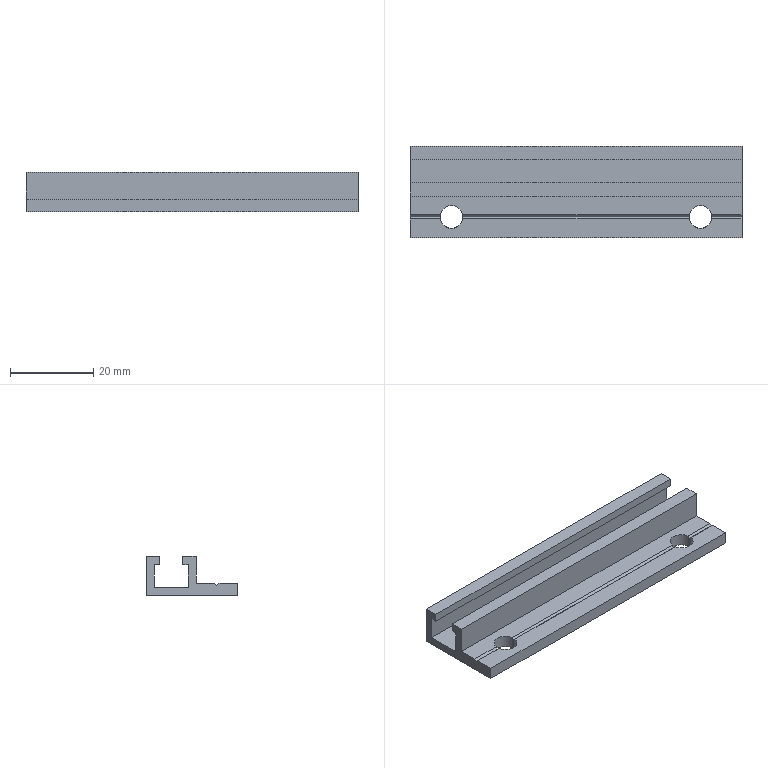Part | STEP file | SENCF5-80 | 1 solid | 27 faces | box 80 x 22 x 9.5 mm | volume 6872 mm3 | plane 23 | cylinder 4 | commonest cylinder face diameters 5.5 x4
STEP:
#1=CARTESIAN_POINT('',(72.704,-0.5,3.));
#2=VERTEX_POINT('',#1);
#3=CARTESIAN_POINT('',(72.75,0.,2.5));
#4=VERTEX_POINT('',#3);
#5=CARTESIAN_POINT('',(72.704,-0.5,3.));
#6=CARTESIAN_POINT('',(72.735,-0.335,2.835));
#7=CARTESIAN_POINT('',(72.75,-0.1678,2.668));
#8=CARTESIAN_POINT('',(72.75,0.,2.5));
#9=(BOUNDED_CURVE()B_SPLINE_CURVE(3,(#5,#6,#7,#8),.UNSPECIFIED.,.F.,.T.)B_SPLINE_CURVE_WITH_KNOTS((4,4),(4.53,4.712),.UNSPECIFIED.)CURVE()GEOMETRIC_REPRESENTATION_ITEM()RATIONAL_B_SPLINE_CURVE((1.,0.9972,0.9972,1.))REPRESENTATION_ITEM(''));
#10=EDGE_CURVE('',#2,#4,#9,.T.);
#11=ORIENTED_EDGE('',*,*,#10,.T.);
#12=CARTESIAN_POINT('',(72.75,0.,0.));
#13=VERTEX_POINT('',#12);
#14=CARTESIAN_POINT('',(72.75,0.,9.5));
#15=DIRECTION('',(0.,0.,-1.));
#16=VECTOR('',#15,1000.);
#17=LINE('',#14,#16);
#18=EDGE_CURVE('',#4,#13,#17,.T.);
#19=ORIENTED_EDGE('',*,*,#18,.T.);
#20=CARTESIAN_POINT('',(67.25,0.,0.));
#21=VERTEX_POINT('',#20);
#22=CARTESIAN_POINT('',(70.,0.,0.));
#23=DIRECTION('',(0.,0.,1.));
#24=DIRECTION('',(1.,0.,0.));
#25=AXIS2_PLACEMENT_3D('',#22,#23,#24);
#26=CIRCLE('',#25,2.75);
#27=EDGE_CURVE('',#21,#13,#26,.T.);
#28=ORIENTED_EDGE('',*,*,#27,.F.);
#29=CARTESIAN_POINT('',(67.25,0.,2.5));
#30=VERTEX_POINT('',#29);
#31=CARTESIAN_POINT('',(67.25,0.,9.5));
#32=DIRECTION('',(0.,0.,-1.));
#33=VECTOR('',#32,1000.);
#34=LINE('',#31,#33);
#35=EDGE_CURVE('',#30,#21,#34,.T.);
#36=ORIENTED_EDGE('',*,*,#35,.F.);
#37=CARTESIAN_POINT('',(67.296,-0.5,3.));
#38=VERTEX_POINT('',#37);
#39=CARTESIAN_POINT('',(67.25,0.,2.5));
#40=CARTESIAN_POINT('',(67.25,-0.1678,2.668));
#41=CARTESIAN_POINT('',(67.265,-0.335,2.835));
#42=CARTESIAN_POINT('',(67.296,-0.5,3.));
#43=(BOUNDED_CURVE()B_SPLINE_CURVE(3,(#39,#40,#41,#42),.UNSPECIFIED.,.F.,.F.)B_SPLINE_CURVE_WITH_KNOTS((4,4),(1.571,1.754),.UNSPECIFIED.)CURVE()GEOMETRIC_REPRESENTATION_ITEM()RATIONAL_B_SPLINE_CURVE((1.,0.9972,0.9972,1.))REPRESENTATION_ITEM(''));
#44=EDGE_CURVE('',#30,#38,#43,.T.);
#45=ORIENTED_EDGE('',*,*,#44,.T.);
#46=CARTESIAN_POINT('',(70.,0.,3.));
#47=DIRECTION('',(0.,0.,1.));
#48=DIRECTION('',(0.,1.,0.));
#49=AXIS2_PLACEMENT_3D('',#46,#47,#48);
#50=CIRCLE('',#49,2.75);
#51=EDGE_CURVE('',#38,#2,#50,.T.);
#52=ORIENTED_EDGE('',*,*,#51,.T.);
#53=EDGE_LOOP('',(#11,#19,#28,#36,#45,#52));
#54=FACE_OUTER_BOUND('',#53,.T.);
#55=CARTESIAN_POINT('',(70.,0.,9.5));
#56=DIRECTION('',(0.,0.,-1.));
#57=DIRECTION('',(-1.,0.,0.));
#58=AXIS2_PLACEMENT_3D('',#55,#56,#57);
#59=CYLINDRICAL_SURFACE('',#58,2.75);
#60=ADVANCED_FACE('',(#54),#59,.F.);
#61=CARTESIAN_POINT('',(12.704,-0.5,3.));
#62=VERTEX_POINT('',#61);
#63=CARTESIAN_POINT('',(12.75,0.,2.5));
#64=VERTEX_POINT('',#63);
#65=CARTESIAN_POINT('',(12.704,-0.5,3.));
#66=CARTESIAN_POINT('',(12.735,-0.335,2.835));
#67=CARTESIAN_POINT('',(12.75,-0.1678,2.668));
#68=CARTESIAN_POINT('',(12.75,0.,2.5));
#69=(BOUNDED_CURVE()B_SPLINE_CURVE(3,(#65,#66,#67,#68),.UNSPECIFIED.,.F.,.F.)B_SPLINE_CURVE_WITH_KNOTS((4,4),(4.53,4.712),.UNSPECIFIED.)CURVE()GEOMETRIC_REPRESENTATION_ITEM()RATIONAL_B_SPLINE_CURVE((1.,0.9972,0.9972,1.))REPRESENTATION_ITEM(''));
#70=EDGE_CURVE('',#62,#64,#69,.T.);
#71=ORIENTED_EDGE('',*,*,#70,.T.);
#72=CARTESIAN_POINT('',(12.75,0.,0.));
#73=VERTEX_POINT('',#72);
#74=CARTESIAN_POINT('',(12.75,0.,9.5));
#75=DIRECTION('',(0.,0.,-1.));
#76=VECTOR('',#75,1000.);
#77=LINE('',#74,#76);
#78=EDGE_CURVE('',#64,#73,#77,.T.);
#79=ORIENTED_EDGE('',*,*,#78,.T.);
#80=CARTESIAN_POINT('',(7.25,0.,0.));
#81=VERTEX_POINT('',#80);
#82=CARTESIAN_POINT('',(10.,0.,0.));
#83=DIRECTION('',(0.,0.,1.));
#84=DIRECTION('',(1.,0.,0.));
#85=AXIS2_PLACEMENT_3D('',#82,#83,#84);
#86=CIRCLE('',#85,2.75);
#87=EDGE_CURVE('',#81,#73,#86,.T.);
#88=ORIENTED_EDGE('',*,*,#87,.F.);
#89=CARTESIAN_POINT('',(7.25,0.,2.5));
#90=VERTEX_POINT('',#89);
#91=CARTESIAN_POINT('',(7.25,0.,9.5));
#92=DIRECTION('',(0.,0.,-1.));
#93=VECTOR('',#92,1000.);
#94=LINE('',#91,#93);
#95=EDGE_CURVE('',#90,#81,#94,.T.);
#96=ORIENTED_EDGE('',*,*,#95,.F.);
#97=CARTESIAN_POINT('',(7.296,-0.5,3.));
#98=VERTEX_POINT('',#97);
#99=CARTESIAN_POINT('',(7.25,0.,2.5));
#100=CARTESIAN_POINT('',(7.25,-0.1678,2.668));
#101=CARTESIAN_POINT('',(7.265,-0.335,2.835));
#102=CARTESIAN_POINT('',(7.296,-0.5,3.));
#103=(BOUNDED_CURVE()B_SPLINE_CURVE(3,(#99,#100,#101,#102),.UNSPECIFIED.,.F.,.F.)B_SPLINE_CURVE_WITH_KNOTS((4,4),(1.571,1.754),.UNSPECIFIED.)CURVE()GEOMETRIC_REPRESENTATION_ITEM()RATIONAL_B_SPLINE_CURVE((1.,0.9972,0.9972,1.))REPRESENTATION_ITEM(''));
#104=EDGE_CURVE('',#90,#98,#103,.T.);
#105=ORIENTED_EDGE('',*,*,#104,.T.);
#106=CARTESIAN_POINT('',(10.,0.,3.));
#107=DIRECTION('',(0.,0.,1.));
#108=DIRECTION('',(0.,1.,0.));
#109=AXIS2_PLACEMENT_3D('',#106,#107,#108);
#110=CIRCLE('',#109,2.75);
#111=EDGE_CURVE('',#98,#62,#110,.T.);
#112=ORIENTED_EDGE('',*,*,#111,.T.);
#113=EDGE_LOOP('',(#71,#79,#88,#96,#105,#112));
#114=FACE_OUTER_BOUND('',#113,.T.);
#115=CARTESIAN_POINT('',(10.,0.,9.5));
#116=DIRECTION('',(0.,0.,-1.));
#117=DIRECTION('',(-1.,0.,0.));
#118=AXIS2_PLACEMENT_3D('',#115,#116,#117);
#119=CYLINDRICAL_SURFACE('',#118,2.75);
#120=ADVANCED_FACE('',(#114),#119,.F.);
#121=CARTESIAN_POINT('',(0.,-5.,0.));
#122=VERTEX_POINT('',#121);
#123=CARTESIAN_POINT('',(0.,17.,0.));
#124=VERTEX_POINT('',#123);
#125=CARTESIAN_POINT('',(0.,-5.,0.));
#126=DIRECTION('',(0.,1.,0.));
#127=VECTOR('',#126,1000.);
#128=LINE('',#125,#127);
#129=EDGE_CURVE('',#122,#124,#128,.T.);
#130=ORIENTED_EDGE('',*,*,#129,.T.);
#131=CARTESIAN_POINT('',(80.,17.,0.));
#132=VERTEX_POINT('',#131);
#133=CARTESIAN_POINT('',(80.,17.,0.));
#134=DIRECTION('',(-1.,0.,0.));
#135=VECTOR('',#134,1000.);
#136=LINE('',#133,#135);
#137=EDGE_CURVE('',#132,#124,#136,.T.);
#138=ORIENTED_EDGE('',*,*,#137,.F.);
#139=CARTESIAN_POINT('',(80.,-5.,0.));
#140=VERTEX_POINT('',#139);
#141=CARTESIAN_POINT('',(80.,-5.,0.));
#142=DIRECTION('',(0.,1.,0.));
#143=VECTOR('',#142,1000.);
#144=LINE('',#141,#143);
#145=EDGE_CURVE('',#140,#132,#144,.T.);
#146=ORIENTED_EDGE('',*,*,#145,.F.);
#147=CARTESIAN_POINT('',(80.,-5.,0.));
#148=DIRECTION('',(-1.,0.,0.));
#149=VECTOR('',#148,1000.);
#150=LINE('',#147,#149);
#151=EDGE_CURVE('',#140,#122,#150,.T.);
#152=ORIENTED_EDGE('',*,*,#151,.T.);
#153=EDGE_LOOP('',(#130,#138,#146,#152));
#154=FACE_OUTER_BOUND('',#153,.T.);
#155=ORIENTED_EDGE('',*,*,#87,.T.);
#156=CARTESIAN_POINT('',(10.,0.,0.));
#157=DIRECTION('',(0.,0.,1.));
#158=DIRECTION('',(1.,0.,0.));
#159=AXIS2_PLACEMENT_3D('',#156,#157,#158);
#160=CIRCLE('',#159,2.75);
#161=EDGE_CURVE('',#73,#81,#160,.T.);
#162=ORIENTED_EDGE('',*,*,#161,.T.);
#163=EDGE_LOOP('',(#155,#162));
#164=FACE_BOUND('',#163,.T.);
#165=ORIENTED_EDGE('',*,*,#27,.T.);
#166=CARTESIAN_POINT('',(70.,0.,0.));
#167=DIRECTION('',(0.,0.,1.));
#168=DIRECTION('',(1.,0.,0.));
#169=AXIS2_PLACEMENT_3D('',#166,#167,#168);
#170=CIRCLE('',#169,2.75);
#171=EDGE_CURVE('',#13,#21,#170,.T.);
#172=ORIENTED_EDGE('',*,*,#171,.T.);
#173=EDGE_LOOP('',(#165,#172));
#174=FACE_BOUND('',#173,.T.);
#175=CARTESIAN_POINT('',(80.,-5.,0.));
#176=DIRECTION('',(0.,0.,1.));
#177=DIRECTION('',(0.,-1.,0.));
#178=AXIS2_PLACEMENT_3D('',#175,#176,#177);
#179=PLANE('',#178);
#180=ADVANCED_FACE('',(#154,#164,#174),#179,.F.);
#181=CARTESIAN_POINT('',(72.704,0.5,3.));
#182=VERTEX_POINT('',#181);
#183=CARTESIAN_POINT('',(67.296,0.5,3.));
#184=VERTEX_POINT('',#183);
#185=CARTESIAN_POINT('',(70.,0.,3.));
#186=DIRECTION('',(0.,0.,1.));
#187=DIRECTION('',(0.,1.,0.));
#188=AXIS2_PLACEMENT_3D('',#185,#186,#187);
#189=CIRCLE('',#188,2.75);
#190=EDGE_CURVE('',#182,#184,#189,.T.);
#191=ORIENTED_EDGE('',*,*,#190,.F.);
#192=CARTESIAN_POINT('',(80.,0.5,3.));
#193=VERTEX_POINT('',#192);
#194=CARTESIAN_POINT('',(80.,0.5,3.));
#195=DIRECTION('',(-1.,0.,0.));
#196=VECTOR('',#195,1000.);
#197=LINE('',#194,#196);
#198=EDGE_CURVE('',#193,#182,#197,.T.);
#199=ORIENTED_EDGE('',*,*,#198,.F.);
#200=CARTESIAN_POINT('',(80.,5.,3.));
#201=VERTEX_POINT('',#200);
#202=CARTESIAN_POINT('',(80.,5.,3.));
#203=DIRECTION('',(0.,-1.,0.));
#204=VECTOR('',#203,1000.);
#205=LINE('',#202,#204);
#206=EDGE_CURVE('',#201,#193,#205,.T.);
#207=ORIENTED_EDGE('',*,*,#206,.F.);
#208=CARTESIAN_POINT('',(0.,5.,3.));
#209=VERTEX_POINT('',#208);
#210=CARTESIAN_POINT('',(80.,5.,3.));
#211=DIRECTION('',(-1.,0.,0.));
#212=VECTOR('',#211,1000.);
#213=LINE('',#210,#212);
#214=EDGE_CURVE('',#201,#209,#213,.T.);
#215=ORIENTED_EDGE('',*,*,#214,.T.);
#216=CARTESIAN_POINT('',(0.,0.5,3.));
#217=VERTEX_POINT('',#216);
#218=CARTESIAN_POINT('',(0.,5.,3.));
#219=DIRECTION('',(0.,-1.,0.));
#220=VECTOR('',#219,1000.);
#221=LINE('',#218,#220);
#222=EDGE_CURVE('',#209,#217,#221,.T.);
#223=ORIENTED_EDGE('',*,*,#222,.T.);
#224=CARTESIAN_POINT('',(7.296,0.5,3.));
#225=VERTEX_POINT('',#224);
#226=CARTESIAN_POINT('',(80.,0.5,3.));
#227=DIRECTION('',(-1.,0.,0.));
#228=VECTOR('',#227,1000.);
#229=LINE('',#226,#228);
#230=EDGE_CURVE('',#225,#217,#229,.T.);
#231=ORIENTED_EDGE('',*,*,#230,.F.);
#232=CARTESIAN_POINT('',(12.704,0.5,3.));
#233=VERTEX_POINT('',#232);
#234=CARTESIAN_POINT('',(10.,0.,3.));
#235=DIRECTION('',(0.,0.,1.));
#236=DIRECTION('',(0.,1.,0.));
#237=AXIS2_PLACEMENT_3D('',#234,#235,#236);
#238=CIRCLE('',#237,2.75);
#239=EDGE_CURVE('',#233,#225,#238,.T.);
#240=ORIENTED_EDGE('',*,*,#239,.F.);
#241=CARTESIAN_POINT('',(80.,0.5,3.));
#242=DIRECTION('',(-1.,0.,0.));
#243=VECTOR('',#242,1000.);
#244=LINE('',#241,#243);
#245=EDGE_CURVE('',#184,#233,#244,.T.);
#246=ORIENTED_EDGE('',*,*,#245,.F.);
#247=EDGE_LOOP('',(#191,#199,#207,#215,#223,#231,#240,#246));
#248=FACE_OUTER_BOUND('',#247,.T.);
#249=CARTESIAN_POINT('',(80.,5.,3.));
#250=DIRECTION('',(0.,0.,-1.));
#251=DIRECTION('',(0.,1.,0.));
#252=AXIS2_PLACEMENT_3D('',#249,#250,#251);
#253=PLANE('',#252);
#254=ADVANCED_FACE('',(#248),#253,.F.);
#255=CARTESIAN_POINT('',(72.75,0.,2.5));
#256=CARTESIAN_POINT('',(72.75,0.1678,2.668));
#257=CARTESIAN_POINT('',(72.735,0.335,2.835));
#258=CARTESIAN_POINT('',(72.704,0.5,3.));
#259=(BOUNDED_CURVE()B_SPLINE_CURVE(3,(#255,#256,#257,#258),.UNSPECIFIED.,.F.,.F.)B_SPLINE_CURVE_WITH_KNOTS((4,4),(1.571,1.754),.UNSPECIFIED.)CURVE()GEOMETRIC_REPRESENTATION_ITEM()RATIONAL_B_SPLINE_CURVE((1.,0.9972,0.9972,1.))REPRESENTATION_ITEM(''));
#260=EDGE_CURVE('',#4,#182,#259,.T.);
#261=ORIENTED_EDGE('',*,*,#260,.F.);
#262=CARTESIAN_POINT('',(80.,0.,2.5));
#263=VERTEX_POINT('',#262);
#264=CARTESIAN_POINT('',(80.,0.,2.5));
#265=DIRECTION('',(-1.,0.,0.));
#266=VECTOR('',#265,1000.);
#267=LINE('',#264,#266);
#268=EDGE_CURVE('',#263,#4,#267,.T.);
#269=ORIENTED_EDGE('',*,*,#268,.F.);
#270=CARTESIAN_POINT('',(80.,0.5,3.));
#271=DIRECTION('',(0.,-0.7071,-0.7071));
#272=VECTOR('',#271,1000.);
#273=LINE('',#270,#272);
#274=EDGE_CURVE('',#193,#263,#273,.T.);
#275=ORIENTED_EDGE('',*,*,#274,.F.);
#276=ORIENTED_EDGE('',*,*,#198,.T.);
#277=EDGE_LOOP('',(#261,#269,#275,#276));
#278=FACE_OUTER_BOUND('',#277,.T.);
#279=CARTESIAN_POINT('',(80.,0.5,3.));
#280=DIRECTION('',(0.,0.7071,-0.7071));
#281=DIRECTION('',(0.,0.7071,0.7071));
#282=AXIS2_PLACEMENT_3D('',#279,#280,#281);
#283=PLANE('',#282);
#284=ADVANCED_FACE('',(#278),#283,.F.);
#285=CARTESIAN_POINT('',(67.296,0.5,3.));
#286=CARTESIAN_POINT('',(67.265,0.335,2.835));
#287=CARTESIAN_POINT('',(67.25,0.1678,2.668));
#288=CARTESIAN_POINT('',(67.25,0.,2.5));
#289=(BOUNDED_CURVE()B_SPLINE_CURVE(3,(#285,#286,#287,#288),.UNSPECIFIED.,.F.,.F.)B_SPLINE_CURVE_WITH_KNOTS((4,4),(4.53,4.712),.UNSPECIFIED.)CURVE()GEOMETRIC_REPRESENTATION_ITEM()RATIONAL_B_SPLINE_CURVE((1.,0.9972,0.9972,1.))REPRESENTATION_ITEM(''));
#290=EDGE_CURVE('',#184,#30,#289,.T.);
#291=ORIENTED_EDGE('',*,*,#290,.F.);
#292=ORIENTED_EDGE('',*,*,#245,.T.);
#293=CARTESIAN_POINT('',(12.75,0.,2.5));
#294=CARTESIAN_POINT('',(12.75,0.1678,2.668));
#295=CARTESIAN_POINT('',(12.735,0.335,2.835));
#296=CARTESIAN_POINT('',(12.704,0.5,3.));
#297=(BOUNDED_CURVE()B_SPLINE_CURVE(3,(#293,#294,#295,#296),.UNSPECIFIED.,.F.,.F.)B_SPLINE_CURVE_WITH_KNOTS((4,4),(1.571,1.754),.UNSPECIFIED.)CURVE()GEOMETRIC_REPRESENTATION_ITEM()RATIONAL_B_SPLINE_CURVE((1.,0.9972,0.9972,1.))REPRESENTATION_ITEM(''));
#298=EDGE_CURVE('',#64,#233,#297,.T.);
#299=ORIENTED_EDGE('',*,*,#298,.F.);
#300=CARTESIAN_POINT('',(80.,0.,2.5));
#301=DIRECTION('',(-1.,0.,0.));
#302=VECTOR('',#301,1000.);
#303=LINE('',#300,#302);
#304=EDGE_CURVE('',#30,#64,#303,.T.);
#305=ORIENTED_EDGE('',*,*,#304,.F.);
#306=EDGE_LOOP('',(#291,#292,#299,#305));
#307=FACE_OUTER_BOUND('',#306,.T.);
#308=CARTESIAN_POINT('',(80.,0.5,3.));
#309=DIRECTION('',(0.,0.7071,-0.7071));
#310=DIRECTION('',(0.,0.7071,0.7071));
#311=AXIS2_PLACEMENT_3D('',#308,#309,#310);
#312=PLANE('',#311);
#313=ADVANCED_FACE('',(#307),#312,.F.);
#314=ORIENTED_EDGE('',*,*,#44,.F.);
#315=ORIENTED_EDGE('',*,*,#304,.T.);
#316=ORIENTED_EDGE('',*,*,#70,.F.);
#317=CARTESIAN_POINT('',(80.,-0.5,3.));
#318=DIRECTION('',(-1.,0.,0.));
#319=VECTOR('',#318,1000.);
#320=LINE('',#317,#319);
#321=EDGE_CURVE('',#38,#62,#320,.T.);
#322=ORIENTED_EDGE('',*,*,#321,.F.);
#323=EDGE_LOOP('',(#314,#315,#316,#322));
#324=FACE_OUTER_BOUND('',#323,.T.);
#325=CARTESIAN_POINT('',(80.,0.,2.5));
#326=DIRECTION('',(0.,-0.7071,-0.7071));
#327=DIRECTION('',(0.,0.7071,-0.7071));
#328=AXIS2_PLACEMENT_3D('',#325,#326,#327);
#329=PLANE('',#328);
#330=ADVANCED_FACE('',(#324),#329,.F.);
#331=ORIENTED_EDGE('',*,*,#10,.F.);
#332=CARTESIAN_POINT('',(80.,-0.5,3.));
#333=VERTEX_POINT('',#332);
#334=CARTESIAN_POINT('',(80.,-0.5,3.));
#335=DIRECTION('',(-1.,0.,0.));
#336=VECTOR('',#335,1000.);
#337=LINE('',#334,#336);
#338=EDGE_CURVE('',#333,#2,#337,.T.);
#339=ORIENTED_EDGE('',*,*,#338,.F.);
#340=CARTESIAN_POINT('',(80.,0.,2.5));
#341=DIRECTION('',(0.,-0.7071,0.7071));
#342=VECTOR('',#341,1000.);
#343=LINE('',#340,#342);
#344=EDGE_CURVE('',#263,#333,#343,.T.);
#345=ORIENTED_EDGE('',*,*,#344,.F.);
#346=ORIENTED_EDGE('',*,*,#268,.T.);
#347=EDGE_LOOP('',(#331,#339,#345,#346));
#348=FACE_OUTER_BOUND('',#347,.T.);
#349=CARTESIAN_POINT('',(80.,0.,2.5));
#350=DIRECTION('',(0.,-0.7071,-0.7071));
#351=DIRECTION('',(0.,0.7071,-0.7071));
#352=AXIS2_PLACEMENT_3D('',#349,#350,#351);
#353=PLANE('',#352);
#354=ADVANCED_FACE('',(#348),#353,.F.);
#355=ORIENTED_EDGE('',*,*,#51,.F.);
#356=ORIENTED_EDGE('',*,*,#321,.T.);
#357=ORIENTED_EDGE('',*,*,#111,.F.);
#358=CARTESIAN_POINT('',(0.,-0.5,3.));
#359=VERTEX_POINT('',#358);
#360=CARTESIAN_POINT('',(80.,-0.5,3.));
#361=DIRECTION('',(-1.,0.,0.));
#362=VECTOR('',#361,1000.);
#363=LINE('',#360,#362);
#364=EDGE_CURVE('',#98,#359,#363,.T.);
#365=ORIENTED_EDGE('',*,*,#364,.T.);
#366=CARTESIAN_POINT('',(0.,-5.,3.));
#367=VERTEX_POINT('',#366);
#368=CARTESIAN_POINT('',(0.,-0.5,3.));
#369=DIRECTION('',(0.,-1.,0.));
#370=VECTOR('',#369,1000.);
#371=LINE('',#368,#370);
#372=EDGE_CURVE('',#359,#367,#371,.T.);
#373=ORIENTED_EDGE('',*,*,#372,.T.);
#374=CARTESIAN_POINT('',(80.,-5.,3.));
#375=VERTEX_POINT('',#374);
#376=CARTESIAN_POINT('',(80.,-5.,3.));
#377=DIRECTION('',(-1.,0.,0.));
#378=VECTOR('',#377,1000.);
#379=LINE('',#376,#378);
#380=EDGE_CURVE('',#375,#367,#379,.T.);
#381=ORIENTED_EDGE('',*,*,#380,.F.);
#382=CARTESIAN_POINT('',(80.,-0.5,3.));
#383=DIRECTION('',(0.,-1.,0.));
#384=VECTOR('',#383,1000.);
#385=LINE('',#382,#384);
#386=EDGE_CURVE('',#333,#375,#385,.T.);
#387=ORIENTED_EDGE('',*,*,#386,.F.);
#388=ORIENTED_EDGE('',*,*,#338,.T.);
#389=EDGE_LOOP('',(#355,#356,#357,#365,#373,#381,#387,#388));
#390=FACE_OUTER_BOUND('',#389,.T.);
#391=CARTESIAN_POINT('',(80.,-0.5,3.));
#392=DIRECTION('',(0.,0.,-1.));
#393=DIRECTION('',(0.,1.,0.));
#394=AXIS2_PLACEMENT_3D('',#391,#392,#393);
#395=PLANE('',#394);
#396=ADVANCED_FACE('',(#390),#395,.F.);
#397=CARTESIAN_POINT('',(7.296,0.5,3.));
#398=CARTESIAN_POINT('',(7.265,0.335,2.835));
#399=CARTESIAN_POINT('',(7.25,0.1678,2.668));
#400=CARTESIAN_POINT('',(7.25,0.,2.5));
#401=(BOUNDED_CURVE()B_SPLINE_CURVE(3,(#397,#398,#399,#400),.UNSPECIFIED.,.F.,.F.)B_SPLINE_CURVE_WITH_KNOTS((4,4),(4.53,4.712),.UNSPECIFIED.)CURVE()GEOMETRIC_REPRESENTATION_ITEM()RATIONAL_B_SPLINE_CURVE((1.,0.9972,0.9972,1.))REPRESENTATION_ITEM(''));
#402=EDGE_CURVE('',#225,#90,#401,.T.);
#403=ORIENTED_EDGE('',*,*,#402,.F.);
#404=ORIENTED_EDGE('',*,*,#230,.T.);
#405=CARTESIAN_POINT('',(0.,0.,2.5));
#406=VERTEX_POINT('',#405);
#407=CARTESIAN_POINT('',(0.,0.5,3.));
#408=DIRECTION('',(0.,-0.7071,-0.7071));
#409=VECTOR('',#408,1000.);
#410=LINE('',#407,#409);
#411=EDGE_CURVE('',#217,#406,#410,.T.);
#412=ORIENTED_EDGE('',*,*,#411,.T.);
#413=CARTESIAN_POINT('',(80.,0.,2.5));
#414=DIRECTION('',(-1.,0.,0.));
#415=VECTOR('',#414,1000.);
#416=LINE('',#413,#415);
#417=EDGE_CURVE('',#90,#406,#416,.T.);
#418=ORIENTED_EDGE('',*,*,#417,.F.);
#419=EDGE_LOOP('',(#403,#404,#412,#418));
#420=FACE_OUTER_BOUND('',#419,.T.);
#421=CARTESIAN_POINT('',(80.,0.5,3.));
#422=DIRECTION('',(0.,0.7071,-0.7071));
#423=DIRECTION('',(0.,0.7071,0.7071));
#424=AXIS2_PLACEMENT_3D('',#421,#422,#423);
#425=PLANE('',#424);
#426=ADVANCED_FACE('',(#420),#425,.F.);
#427=ORIENTED_EDGE('',*,*,#104,.F.);
#428=ORIENTED_EDGE('',*,*,#417,.T.);
#429=CARTESIAN_POINT('',(0.,0.,2.5));
#430=DIRECTION('',(0.,-0.7071,0.7071));
#431=VECTOR('',#430,1000.);
#432=LINE('',#429,#431);
#433=EDGE_CURVE('',#406,#359,#432,.T.);
#434=ORIENTED_EDGE('',*,*,#433,.T.);
#435=ORIENTED_EDGE('',*,*,#364,.F.);
#436=EDGE_LOOP('',(#427,#428,#434,#435));
#437=FACE_OUTER_BOUND('',#436,.T.);
#438=CARTESIAN_POINT('',(80.,0.,2.5));
#439=DIRECTION('',(0.,-0.7071,-0.7071));
#440=DIRECTION('',(0.,0.7071,-0.7071));
#441=AXIS2_PLACEMENT_3D('',#438,#439,#440);
#442=PLANE('',#441);
#443=ADVANCED_FACE('',(#437),#442,.F.);
#444=CARTESIAN_POINT('',(0.,17.,9.5));
#445=VERTEX_POINT('',#444);
#446=CARTESIAN_POINT('',(0.,17.,0.));
#447=DIRECTION('',(0.,0.,1.));
#448=VECTOR('',#447,1000.);
#449=LINE('',#446,#448);
#450=EDGE_CURVE('',#124,#445,#449,.T.);
#451=ORIENTED_EDGE('',*,*,#450,.T.);
#452=CARTESIAN_POINT('',(80.,17.,9.5));
#453=VERTEX_POINT('',#452);
#454=CARTESIAN_POINT('',(80.,17.,9.5));
#455=DIRECTION('',(-1.,0.,0.));
#456=VECTOR('',#455,1000.);
#457=LINE('',#454,#456);
#458=EDGE_CURVE('',#453,#445,#457,.T.);
#459=ORIENTED_EDGE('',*,*,#458,.F.);
#460=CARTESIAN_POINT('',(80.,17.,0.));
#461=DIRECTION('',(0.,0.,1.));
#462=VECTOR('',#461,1000.);
#463=LINE('',#460,#462);
#464=EDGE_CURVE('',#132,#453,#463,.T.);
#465=ORIENTED_EDGE('',*,*,#464,.F.);
#466=ORIENTED_EDGE('',*,*,#137,.T.);
#467=EDGE_LOOP('',(#451,#459,#465,#466));
#468=FACE_OUTER_BOUND('',#467,.T.);
#469=CARTESIAN_POINT('',(80.,17.,0.));
#470=DIRECTION('',(0.,-1.,0.));
#471=DIRECTION('',(0.,0.,-1.));
#472=AXIS2_PLACEMENT_3D('',#469,#470,#471);
#473=PLANE('',#472);
#474=ADVANCED_FACE('',(#468),#473,.F.);
#475=CARTESIAN_POINT('',(0.,13.75,9.5));
#476=VERTEX_POINT('',#475);
#477=CARTESIAN_POINT('',(0.,17.,9.5));
#478=DIRECTION('',(0.,-1.,0.));
#479=VECTOR('',#478,1000.);
#480=LINE('',#477,#479);
#481=EDGE_CURVE('',#445,#476,#480,.T.);
#482=ORIENTED_EDGE('',*,*,#481,.T.);
#483=CARTESIAN_POINT('',(80.,13.75,9.5));
#484=VERTEX_POINT('',#483);
#485=CARTESIAN_POINT('',(80.,13.75,9.5));
#486=DIRECTION('',(-1.,0.,0.));
#487=VECTOR('',#486,1000.);
#488=LINE('',#485,#487);
#489=EDGE_CURVE('',#484,#476,#488,.T.);
#490=ORIENTED_EDGE('',*,*,#489,.F.);
#491=CARTESIAN_POINT('',(80.,17.,9.5));
#492=DIRECTION('',(0.,-1.,0.));
#493=VECTOR('',#492,1000.);
#494=LINE('',#491,#493);
#495=EDGE_CURVE('',#453,#484,#494,.T.);
#496=ORIENTED_EDGE('',*,*,#495,.F.);
#497=ORIENTED_EDGE('',*,*,#458,.T.);
#498=EDGE_LOOP('',(#482,#490,#496,#497));
#499=FACE_OUTER_BOUND('',#498,.T.);
#500=CARTESIAN_POINT('',(80.,17.,9.5));
#501=DIRECTION('',(0.,0.,-1.));
#502=DIRECTION('',(0.,1.,0.));
#503=AXIS2_PLACEMENT_3D('',#500,#501,#502);
#504=PLANE('',#503);
#505=ADVANCED_FACE('',(#499),#504,.F.);
#506=CARTESIAN_POINT('',(0.,13.75,7.5));
#507=VERTEX_POINT('',#506);
#508=CARTESIAN_POINT('',(0.,13.75,9.5));
#509=DIRECTION('',(0.,0.,-1.));
#510=VECTOR('',#509,1000.);
#511=LINE('',#508,#510);
#512=EDGE_CURVE('',#476,#507,#511,.T.);
#513=ORIENTED_EDGE('',*,*,#512,.T.);
#514=CARTESIAN_POINT('',(80.,13.75,7.5));
#515=VERTEX_POINT('',#514);
#516=CARTESIAN_POINT('',(80.,13.75,7.5));
#517=DIRECTION('',(-1.,0.,0.));
#518=VECTOR('',#517,1000.);
#519=LINE('',#516,#518);
#520=EDGE_CURVE('',#515,#507,#519,.T.);
#521=ORIENTED_EDGE('',*,*,#520,.F.);
#522=CARTESIAN_POINT('',(80.,13.75,9.5));
#523=DIRECTION('',(0.,0.,-1.));
#524=VECTOR('',#523,1000.);
#525=LINE('',#522,#524);
#526=EDGE_CURVE('',#484,#515,#525,.T.);
#527=ORIENTED_EDGE('',*,*,#526,.F.);
#528=ORIENTED_EDGE('',*,*,#489,.T.);
#529=EDGE_LOOP('',(#513,#521,#527,#528));
#530=FACE_OUTER_BOUND('',#529,.T.);
#531=CARTESIAN_POINT('',(80.,13.75,9.5));
#532=DIRECTION('',(0.,1.,0.));
#533=DIRECTION('',(0.,0.,1.));
#534=AXIS2_PLACEMENT_3D('',#531,#532,#533);
#535=PLANE('',#534);
#536=ADVANCED_FACE('',(#530),#535,.F.);
#537=CARTESIAN_POINT('',(0.,15.1,7.5));
#538=VERTEX_POINT('',#537);
#539=CARTESIAN_POINT('',(0.,13.75,7.5));
#540=DIRECTION('',(0.,1.,0.));
#541=VECTOR('',#540,1000.);
#542=LINE('',#539,#541);
#543=EDGE_CURVE('',#507,#538,#542,.T.);
#544=ORIENTED_EDGE('',*,*,#543,.T.);
#545=CARTESIAN_POINT('',(80.,15.1,7.5));
#546=VERTEX_POINT('',#545);
#547=CARTESIAN_POINT('',(80.,15.1,7.5));
#548=DIRECTION('',(-1.,0.,0.));
#549=VECTOR('',#548,1000.);
#550=LINE('',#547,#549);
#551=EDGE_CURVE('',#546,#538,#550,.T.);
#552=ORIENTED_EDGE('',*,*,#551,.F.);
#553=CARTESIAN_POINT('',(80.,13.75,7.5));
#554=DIRECTION('',(0.,1.,0.));
#555=VECTOR('',#554,1000.);
#556=LINE('',#553,#555);
#557=EDGE_CURVE('',#515,#546,#556,.T.);
#558=ORIENTED_EDGE('',*,*,#557,.F.);
#559=ORIENTED_EDGE('',*,*,#520,.T.);
#560=EDGE_LOOP('',(#544,#552,#558,#559));
#561=FACE_OUTER_BOUND('',#560,.T.);
#562=CARTESIAN_POINT('',(80.,13.75,7.5));
#563=DIRECTION('',(0.,0.,1.));
#564=DIRECTION('',(1.,0.,0.));
#565=AXIS2_PLACEMENT_3D('',#562,#563,#564);
#566=PLANE('',#565);
#567=ADVANCED_FACE('',(#561),#566,.F.);
#568=CARTESIAN_POINT('',(0.,15.1,2.));
#569=VERTEX_POINT('',#568);
#570=CARTESIAN_POINT('',(0.,15.1,7.5));
#571=DIRECTION('',(0.,0.,-1.));
#572=VECTOR('',#571,1000.);
#573=LINE('',#570,#572);
#574=EDGE_CURVE('',#538,#569,#573,.T.);
#575=ORIENTED_EDGE('',*,*,#574,.T.);
#576=CARTESIAN_POINT('',(80.,15.1,2.));
#577=VERTEX_POINT('',#576);
#578=CARTESIAN_POINT('',(80.,15.1,2.));
#579=DIRECTION('',(-1.,0.,0.));
#580=VECTOR('',#579,1000.);
#581=LINE('',#578,#580);
#582=EDGE_CURVE('',#577,#569,#581,.T.);
#583=ORIENTED_EDGE('',*,*,#582,.F.);
#584=CARTESIAN_POINT('',(80.,15.1,7.5));
#585=DIRECTION('',(0.,0.,-1.));
#586=VECTOR('',#585,1000.);
#587=LINE('',#584,#586);
#588=EDGE_CURVE('',#546,#577,#587,.T.);
#589=ORIENTED_EDGE('',*,*,#588,.F.);
#590=ORIENTED_EDGE('',*,*,#551,.T.);
#591=EDGE_LOOP('',(#575,#583,#589,#590));
#592=FACE_OUTER_BOUND('',#591,.T.);
#593=CARTESIAN_POINT('',(80.,15.1,7.5));
#594=DIRECTION('',(0.,1.,0.));
#595=DIRECTION('',(0.,0.,1.));
#596=AXIS2_PLACEMENT_3D('',#593,#594,#595);
#597=PLANE('',#596);
#598=ADVANCED_FACE('',(#592),#597,.F.);
#599=CARTESIAN_POINT('',(0.,6.9,2.));
#600=VERTEX_POINT('',#599);
#601=CARTESIAN_POINT('',(0.,15.1,2.));
#602=DIRECTION('',(0.,-1.,0.));
#603=VECTOR('',#602,1000.);
#604=LINE('',#601,#603);
#605=EDGE_CURVE('',#569,#600,#604,.T.);
#606=ORIENTED_EDGE('',*,*,#605,.T.);
#607=CARTESIAN_POINT('',(80.,6.9,2.));
#608=VERTEX_POINT('',#607);
#609=CARTESIAN_POINT('',(80.,6.9,2.));
#610=DIRECTION('',(-1.,0.,0.));
#611=VECTOR('',#610,1000.);
#612=LINE('',#609,#611);
#613=EDGE_CURVE('',#608,#600,#612,.T.);
#614=ORIENTED_EDGE('',*,*,#613,.F.);
#615=CARTESIAN_POINT('',(80.,15.1,2.));
#616=DIRECTION('',(0.,-1.,0.));
#617=VECTOR('',#616,1000.);
#618=LINE('',#615,#617);
#619=EDGE_CURVE('',#577,#608,#618,.T.);
#620=ORIENTED_EDGE('',*,*,#619,.F.);
#621=ORIENTED_EDGE('',*,*,#582,.T.);
#622=EDGE_LOOP('',(#606,#614,#620,#621));
#623=FACE_OUTER_BOUND('',#622,.T.);
#624=CARTESIAN_POINT('',(80.,15.1,2.));
#625=DIRECTION('',(0.,0.,-1.));
#626=DIRECTION('',(0.,1.,0.));
#627=AXIS2_PLACEMENT_3D('',#624,#625,#626);
#628=PLANE('',#627);
#629=ADVANCED_FACE('',(#623),#628,.F.);
#630=CARTESIAN_POINT('',(0.,6.9,7.5));
#631=VERTEX_POINT('',#630);
#632=CARTESIAN_POINT('',(0.,6.9,2.));
#633=DIRECTION('',(0.,0.,1.));
#634=VECTOR('',#633,1000.);
#635=LINE('',#632,#634);
#636=EDGE_CURVE('',#600,#631,#635,.T.);
#637=ORIENTED_EDGE('',*,*,#636,.T.);
#638=CARTESIAN_POINT('',(80.,6.9,7.5));
#639=VERTEX_POINT('',#638);
#640=CARTESIAN_POINT('',(80.,6.9,7.5));
#641=DIRECTION('',(-1.,0.,0.));
#642=VECTOR('',#641,1000.);
#643=LINE('',#640,#642);
#644=EDGE_CURVE('',#639,#631,#643,.T.);
#645=ORIENTED_EDGE('',*,*,#644,.F.);
#646=CARTESIAN_POINT('',(80.,6.9,2.));
#647=DIRECTION('',(0.,0.,1.));
#648=VECTOR('',#647,1000.);
#649=LINE('',#646,#648);
#650=EDGE_CURVE('',#608,#639,#649,.T.);
#651=ORIENTED_EDGE('',*,*,#650,.F.);
#652=ORIENTED_EDGE('',*,*,#613,.T.);
#653=EDGE_LOOP('',(#637,#645,#651,#652));
#654=FACE_OUTER_BOUND('',#653,.T.);
#655=CARTESIAN_POINT('',(80.,6.9,2.));
#656=DIRECTION('',(0.,-1.,0.));
#657=DIRECTION('',(0.,0.,-1.));
#658=AXIS2_PLACEMENT_3D('',#655,#656,#657);
#659=PLANE('',#658);
#660=ADVANCED_FACE('',(#654),#659,.F.);
#661=CARTESIAN_POINT('',(0.,8.25,7.5));
#662=VERTEX_POINT('',#661);
#663=CARTESIAN_POINT('',(0.,6.9,7.5));
#664=DIRECTION('',(0.,1.,0.));
#665=VECTOR('',#664,1000.);
#666=LINE('',#663,#665);
#667=EDGE_CURVE('',#631,#662,#666,.T.);
#668=ORIENTED_EDGE('',*,*,#667,.T.);
#669=CARTESIAN_POINT('',(80.,8.25,7.5));
#670=VERTEX_POINT('',#669);
#671=CARTESIAN_POINT('',(80.,8.25,7.5));
#672=DIRECTION('',(-1.,0.,0.));
#673=VECTOR('',#672,1000.);
#674=LINE('',#671,#673);
#675=EDGE_CURVE('',#670,#662,#674,.T.);
#676=ORIENTED_EDGE('',*,*,#675,.F.);
#677=CARTESIAN_POINT('',(80.,6.9,7.5));
#678=DIRECTION('',(0.,1.,0.));
#679=VECTOR('',#678,1000.);
#680=LINE('',#677,#679);
#681=EDGE_CURVE('',#639,#670,#680,.T.);
#682=ORIENTED_EDGE('',*,*,#681,.F.);
#683=ORIENTED_EDGE('',*,*,#644,.T.);
#684=EDGE_LOOP('',(#668,#676,#682,#683));
#685=FACE_OUTER_BOUND('',#684,.T.);
#686=CARTESIAN_POINT('',(80.,6.9,7.5));
#687=DIRECTION('',(0.,0.,1.));
#688=DIRECTION('',(1.,0.,0.));
#689=AXIS2_PLACEMENT_3D('',#686,#687,#688);
#690=PLANE('',#689);
#691=ADVANCED_FACE('',(#685),#690,.F.);
#692=CARTESIAN_POINT('',(0.,8.25,9.5));
#693=VERTEX_POINT('',#692);
#694=CARTESIAN_POINT('',(0.,8.25,7.5));
#695=DIRECTION('',(0.,0.,1.));
#696=VECTOR('',#695,1000.);
#697=LINE('',#694,#696);
#698=EDGE_CURVE('',#662,#693,#697,.T.);
#699=ORIENTED_EDGE('',*,*,#698,.T.);
#700=CARTESIAN_POINT('',(80.,8.25,9.5));
#701=VERTEX_POINT('',#700);
#702=CARTESIAN_POINT('',(80.,8.25,9.5));
#703=DIRECTION('',(-1.,0.,0.));
#704=VECTOR('',#703,1000.);
#705=LINE('',#702,#704);
#706=EDGE_CURVE('',#701,#693,#705,.T.);
#707=ORIENTED_EDGE('',*,*,#706,.F.);
#708=CARTESIAN_POINT('',(80.,8.25,7.5));
#709=DIRECTION('',(0.,0.,1.));
#710=VECTOR('',#709,1000.);
#711=LINE('',#708,#710);
#712=EDGE_CURVE('',#670,#701,#711,.T.);
#713=ORIENTED_EDGE('',*,*,#712,.F.);
#714=ORIENTED_EDGE('',*,*,#675,.T.);
#715=EDGE_LOOP('',(#699,#707,#713,#714));
#716=FACE_OUTER_BOUND('',#715,.T.);
#717=CARTESIAN_POINT('',(80.,8.25,7.5));
#718=DIRECTION('',(0.,-1.,0.));
#719=DIRECTION('',(0.,0.,-1.));
#720=AXIS2_PLACEMENT_3D('',#717,#718,#719);
#721=PLANE('',#720);
#722=ADVANCED_FACE('',(#716),#721,.F.);
#723=CARTESIAN_POINT('',(0.,5.,9.5));
#724=VERTEX_POINT('',#723);
#725=CARTESIAN_POINT('',(0.,8.25,9.5));
#726=DIRECTION('',(0.,-1.,0.));
#727=VECTOR('',#726,1000.);
#728=LINE('',#725,#727);
#729=EDGE_CURVE('',#693,#724,#728,.T.);
#730=ORIENTED_EDGE('',*,*,#729,.T.);
#731=CARTESIAN_POINT('',(80.,5.,9.5));
#732=VERTEX_POINT('',#731);
#733=CARTESIAN_POINT('',(80.,5.,9.5));
#734=DIRECTION('',(-1.,0.,0.));
#735=VECTOR('',#734,1000.);
#736=LINE('',#733,#735);
#737=EDGE_CURVE('',#732,#724,#736,.T.);
#738=ORIENTED_EDGE('',*,*,#737,.F.);
#739=CARTESIAN_POINT('',(80.,8.25,9.5));
#740=DIRECTION('',(0.,-1.,0.));
#741=VECTOR('',#740,1000.);
#742=LINE('',#739,#741);
#743=EDGE_CURVE('',#701,#732,#742,.T.);
#744=ORIENTED_EDGE('',*,*,#743,.F.);
#745=ORIENTED_EDGE('',*,*,#706,.T.);
#746=EDGE_LOOP('',(#730,#738,#744,#745));
#747=FACE_OUTER_BOUND('',#746,.T.);
#748=CARTESIAN_POINT('',(80.,8.25,9.5));
#749=DIRECTION('',(0.,0.,-1.));
#750=DIRECTION('',(-1.,0.,0.));
#751=AXIS2_PLACEMENT_3D('',#748,#749,#750);
#752=PLANE('',#751);
#753=ADVANCED_FACE('',(#747),#752,.F.);
#754=CARTESIAN_POINT('',(0.,5.,9.5));
#755=DIRECTION('',(0.,0.,-1.));
#756=VECTOR('',#755,1000.);
#757=LINE('',#754,#756);
#758=EDGE_CURVE('',#724,#209,#757,.T.);
#759=ORIENTED_EDGE('',*,*,#758,.T.);
#760=ORIENTED_EDGE('',*,*,#214,.F.);
#761=CARTESIAN_POINT('',(80.,5.,9.5));
#762=DIRECTION('',(0.,0.,-1.));
#763=VECTOR('',#762,1000.);
#764=LINE('',#761,#763);
#765=EDGE_CURVE('',#732,#201,#764,.T.);
#766=ORIENTED_EDGE('',*,*,#765,.F.);
#767=ORIENTED_EDGE('',*,*,#737,.T.);
#768=EDGE_LOOP('',(#759,#760,#766,#767));
#769=FACE_OUTER_BOUND('',#768,.T.);
#770=CARTESIAN_POINT('',(80.,5.,9.5));
#771=DIRECTION('',(0.,1.,0.));
#772=DIRECTION('',(0.,0.,1.));
#773=AXIS2_PLACEMENT_3D('',#770,#771,#772);
#774=PLANE('',#773);
#775=ADVANCED_FACE('',(#769),#774,.F.);
#776=CARTESIAN_POINT('',(0.,-5.,3.));
#777=DIRECTION('',(0.,0.,-1.));
#778=VECTOR('',#777,1000.);
#779=LINE('',#776,#778);
#780=EDGE_CURVE('',#367,#122,#779,.T.);
#781=ORIENTED_EDGE('',*,*,#780,.T.);
#782=ORIENTED_EDGE('',*,*,#151,.F.);
#783=CARTESIAN_POINT('',(80.,-5.,3.));
#784=DIRECTION('',(0.,0.,-1.));
#785=VECTOR('',#784,1000.);
#786=LINE('',#783,#785);
#787=EDGE_CURVE('',#375,#140,#786,.T.);
#788=ORIENTED_EDGE('',*,*,#787,.F.);
#789=ORIENTED_EDGE('',*,*,#380,.T.);
#790=EDGE_LOOP('',(#781,#782,#788,#789));
#791=FACE_OUTER_BOUND('',#790,.T.);
#792=CARTESIAN_POINT('',(80.,-5.,3.));
#793=DIRECTION('',(0.,1.,0.));
#794=DIRECTION('',(0.,0.,1.));
#795=AXIS2_PLACEMENT_3D('',#792,#793,#794);
#796=PLANE('',#795);
#797=ADVANCED_FACE('',(#791),#796,.F.);
#798=ORIENTED_EDGE('',*,*,#145,.T.);
#799=ORIENTED_EDGE('',*,*,#464,.T.);
#800=ORIENTED_EDGE('',*,*,#495,.T.);
#801=ORIENTED_EDGE('',*,*,#526,.T.);
#802=ORIENTED_EDGE('',*,*,#557,.T.);
#803=ORIENTED_EDGE('',*,*,#588,.T.);
#804=ORIENTED_EDGE('',*,*,#619,.T.);
#805=ORIENTED_EDGE('',*,*,#650,.T.);
#806=ORIENTED_EDGE('',*,*,#681,.T.);
#807=ORIENTED_EDGE('',*,*,#712,.T.);
#808=ORIENTED_EDGE('',*,*,#743,.T.);
#809=ORIENTED_EDGE('',*,*,#765,.T.);
#810=ORIENTED_EDGE('',*,*,#206,.T.);
#811=ORIENTED_EDGE('',*,*,#274,.T.);
#812=ORIENTED_EDGE('',*,*,#344,.T.);
#813=ORIENTED_EDGE('',*,*,#386,.T.);
#814=ORIENTED_EDGE('',*,*,#787,.T.);
#815=EDGE_LOOP('',(#798,#799,#800,#801,#802,#803,#804,#805,#806,#807,#808,#809,#810,#811,#812,#813,#814));
#816=FACE_OUTER_BOUND('',#815,.T.);
#817=CARTESIAN_POINT('',(80.,0.,0.));
#818=DIRECTION('',(1.,0.,0.));
#819=DIRECTION('',(0.,0.,-1.));
#820=AXIS2_PLACEMENT_3D('',#817,#818,#819);
#821=PLANE('',#820);
#822=ADVANCED_FACE('',(#816),#821,.T.);
#823=ORIENTED_EDGE('',*,*,#129,.F.);
#824=ORIENTED_EDGE('',*,*,#780,.F.);
#825=ORIENTED_EDGE('',*,*,#372,.F.);
#826=ORIENTED_EDGE('',*,*,#433,.F.);
#827=ORIENTED_EDGE('',*,*,#411,.F.);
#828=ORIENTED_EDGE('',*,*,#222,.F.);
#829=ORIENTED_EDGE('',*,*,#758,.F.);
#830=ORIENTED_EDGE('',*,*,#729,.F.);
#831=ORIENTED_EDGE('',*,*,#698,.F.);
#832=ORIENTED_EDGE('',*,*,#667,.F.);
#833=ORIENTED_EDGE('',*,*,#636,.F.);
#834=ORIENTED_EDGE('',*,*,#605,.F.);
#835=ORIENTED_EDGE('',*,*,#574,.F.);
#836=ORIENTED_EDGE('',*,*,#543,.F.);
#837=ORIENTED_EDGE('',*,*,#512,.F.);
#838=ORIENTED_EDGE('',*,*,#481,.F.);
#839=ORIENTED_EDGE('',*,*,#450,.F.);
#840=EDGE_LOOP('',(#823,#824,#825,#826,#827,#828,#829,#830,#831,#832,#833,#834,#835,#836,#837,#838,#839));
#841=FACE_OUTER_BOUND('',#840,.T.);
#842=CARTESIAN_POINT('',(0.,0.,0.));
#843=DIRECTION('',(1.,0.,0.));
#844=DIRECTION('',(0.,0.,-1.));
#845=AXIS2_PLACEMENT_3D('',#842,#843,#844);
#846=PLANE('',#845);
#847=ADVANCED_FACE('',(#841),#846,.F.);
#848=ORIENTED_EDGE('',*,*,#78,.F.);
#849=ORIENTED_EDGE('',*,*,#298,.T.);
#850=ORIENTED_EDGE('',*,*,#239,.T.);
#851=ORIENTED_EDGE('',*,*,#402,.T.);
#852=ORIENTED_EDGE('',*,*,#95,.T.);
#853=ORIENTED_EDGE('',*,*,#161,.F.);
#854=EDGE_LOOP('',(#848,#849,#850,#851,#852,#853));
#855=FACE_OUTER_BOUND('',#854,.T.);
#856=CARTESIAN_POINT('',(10.,0.,9.5));
#857=DIRECTION('',(0.,0.,-1.));
#858=DIRECTION('',(-1.,0.,0.));
#859=AXIS2_PLACEMENT_3D('',#856,#857,#858);
#860=CYLINDRICAL_SURFACE('',#859,2.75);
#861=ADVANCED_FACE('',(#855),#860,.F.);
#862=ORIENTED_EDGE('',*,*,#18,.F.);
#863=ORIENTED_EDGE('',*,*,#260,.T.);
#864=ORIENTED_EDGE('',*,*,#190,.T.);
#865=ORIENTED_EDGE('',*,*,#290,.T.);
#866=ORIENTED_EDGE('',*,*,#35,.T.);
#867=ORIENTED_EDGE('',*,*,#171,.F.);
#868=EDGE_LOOP('',(#862,#863,#864,#865,#866,#867));
#869=FACE_OUTER_BOUND('',#868,.T.);
#870=CARTESIAN_POINT('',(70.,0.,9.5));
#871=DIRECTION('',(0.,0.,-1.));
#872=DIRECTION('',(-1.,0.,0.));
#873=AXIS2_PLACEMENT_3D('',#870,#871,#872);
#874=CYLINDRICAL_SURFACE('',#873,2.75);
#875=ADVANCED_FACE('',(#869),#874,.F.);
#876=CLOSED_SHELL('',(#60,#120,#180,#254,#284,#313,#330,#354,#396,#426,#443,#474,#505,#536,#567,#598,#629,#660,#691,#722,#753,#775,#797,#822,#847,#861,#875));
#877=MANIFOLD_SOLID_BREP('',#876);
#878=CARTESIAN_POINT('',(0.,0.,0.));
#879=DIRECTION('',(0.,0.,1.));
#880=DIRECTION('',(1.,0.,0.));
#881=AXIS2_PLACEMENT_3D('',#878,#879,#880);
#882=(LENGTH_UNIT()NAMED_UNIT(*)SI_UNIT(.MILLI.,.METRE.));
#883=UNCERTAINTY_MEASURE_WITH_UNIT(LENGTH_MEASURE(0.00001),#882,'','');
#884=(NAMED_UNIT(*)PLANE_ANGLE_UNIT()SI_UNIT($,.RADIAN.));
#885=(NAMED_UNIT(*)SI_UNIT($,.STERADIAN.)SOLID_ANGLE_UNIT());
#886=(GEOMETRIC_REPRESENTATION_CONTEXT(3)GLOBAL_UNCERTAINTY_ASSIGNED_CONTEXT((#883))GLOBAL_UNIT_ASSIGNED_CONTEXT((#882,#884,#885))REPRESENTATION_CONTEXT('',''));
#887=ADVANCED_BREP_SHAPE_REPRESENTATION('',(#877,#881),#886);